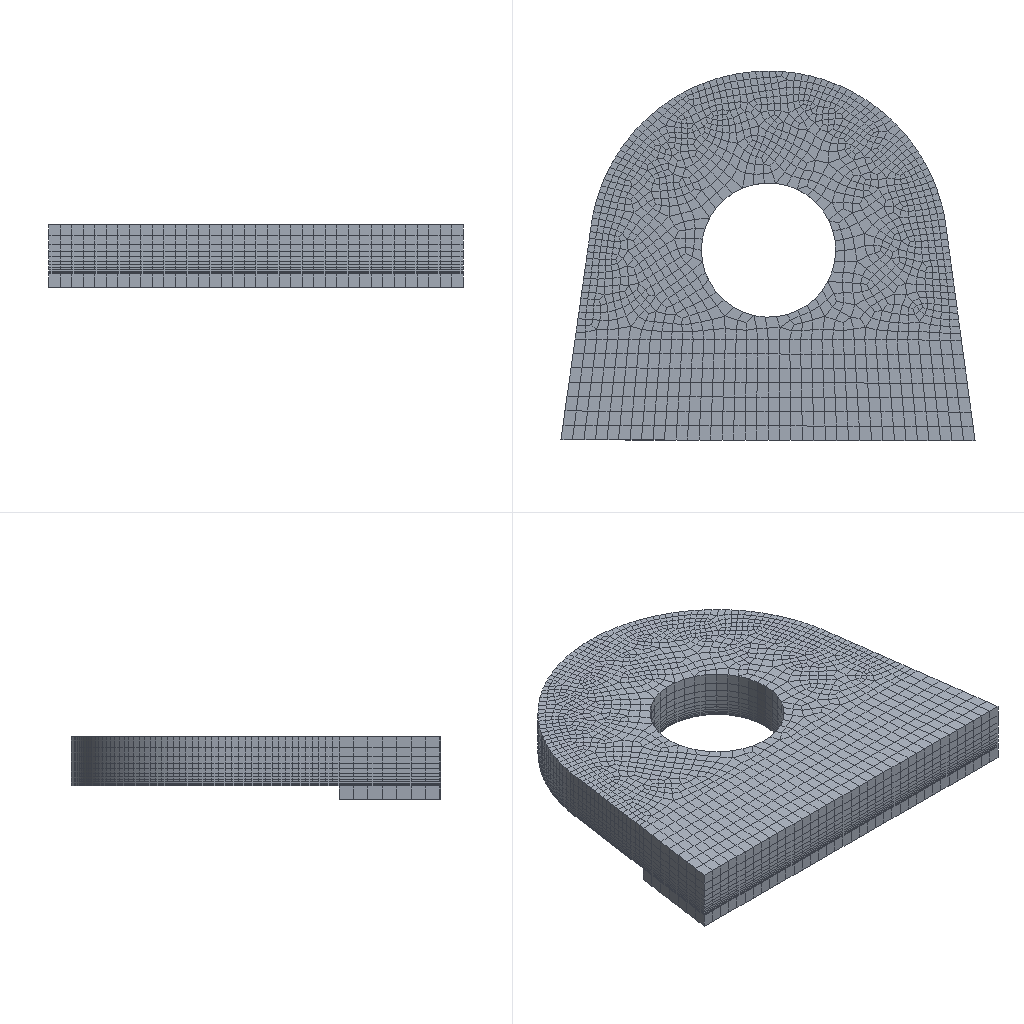Simulation study | abaqus
Set-up summary:
category,name,step,type,value,unit,region
solver,abaqus
solver,version,,,Abaqus/Explicit 2020
units,not stated in the deck,,not stated
analysis,deck,,transient,transient
load_step,Step-1,Step-1,transient
load_step,requested,,,1
mesh,nodes,,,20642
mesh,elements,,,17959
element_type,R3D3,,rigid,72
element_type,R3D4,,rigid,1311
element_type,C3D8R,,solid,16576
load,load commands in deck,,count,2
bc,support commands in deck,,count,7
material,MATERIAL-1,,in results
check,setup vs results,,match,"per instance, exact: element labels, types and connectivity; labels of the nodes the elements use; coordinates of those nodes at SINGLE_PRECISION in 1 of 2 instance(s)"
Abaqus input file, long lists of numbers shortened:
*Heading
** Job name: Job-1 Model name: Model-1
** Generated by: Abaqus/CAE 2020
*Preprint, echo=NO, model=NO, history=NO, contact=NO
**
** PARTS
**
*Part, name=work-1
*Node
      1,  -42.966,   51.411,  -25.061
      2,  -42.139,   50.996,  -24.866
** (1347 more lines like these left out)
*Element, type=R3D4
 1,   1,  25, 357,  62
 2,  25,   2,  26, 357
** (1309 more lines like these left out)
*Element, type=R3D3
39, 75,  5, 63
55,   9,  76, 143
** (70 more lines like these left out)
*Node
   1350,  -37.888,   63.4,  -26.953
*Nset, nset=work-1-RefPt_, internal
1350,
*Elset, elset=work-1, generate
    1,  1383,     1
*End Part
**
*Part, name=work-2
*Node
      1,  -25.624,   43.005,  -23.952
      2,  -27.048,   38.691,  -23.952
** (19290 more lines like these left out)
*Element, type=C3D8R
  1, 112, 568, 778,  43,   1,  19,  30,   4
  2, 568, 569, 779, 778,  19,  20,  29,  30
** (16574 more lines like these left out)
*Nset, nset=Set-1, generate
     1,  19292,      1
*Elset, elset=Set-1, generate
     1,  16576,      1
** Section: Section-1
*Solid Section, elset=Set-1, material=Material-1
,
*End Part
**
**
** ASSEMBLY
**
*Assembly, name=Assembly
**
*Instance, name=work-1-1, part=work-1
41.272, -22.918,    25.552
41.272, -22.918,    25.552, 41.272, -22.918, 26.552, 26.
*End Instance
**
*Instance, name=work-2-1, part=work-2
41.272, -22.918,    24.552
41.272, -22.918,    24.552, 41.272, -22.918, 25.552, 26.
*End Instance
**
*Nset, nset=Set-2, instance=work-2-1
    2,    3,    5,    6,   15,   16,  113,  114,  115,  116,  117,  118,  119,  120,  121,  122
  123,  124,  125,  126,  127,  128,  129,  130,  131,  132,  133,  134,  135,  136,  137,  138
** (29 more lines like these left out)
*Elset, elset=Set-2, instance=work-2-1
     7,    14,    21,    28,    35,    42,    49,    56,    63,    70,    77,    84,    91,    98,   105,   112
   119,   126,   133,   140,   147,   154,   161,   168,   175,   182,   189,   196,   203,   210,   217,   224
** (25 more lines like these left out)
*Nset, nset=Set-3, instance=work-1-1
 1350,
*Nset, nset=s_Set-1, instance=work-2-1
     1,     2,     5,     8,     9,    10,    11,    12,    13,    14,    15,    16,    17,    18,    19,    20
    21,    22,    23,    24,    31,    32,    33,    34,    35,    36,    78,    79,    80,    81,    82,    83
** (1186 more lines like these left out)
*Elset, elset=s_Set-1, instance=work-2-1, generate
   253,  16576,      1
*Elset, elset=_m_Surf-1_SPOS, internal, instance=work-1-1, generate
    1,  1383,     1
*Surface, type=ELEMENT, name=m_Surf-1
_m_Surf-1_SPOS, SPOS
*Surface, type=NODE, name=s_Set-1_CNS_, internal
s_Set-1, 1.
*Rigid Body, ref node=work-1-1.work-1-RefPt_, elset=work-1-1.work-1
*End Assembly
**
** MATERIALS
**
*Material, name=Material-1
*Damage Initiation, criterion=SHEAR
 0.01,0.,0.
*Damage Evolution, type=DISPLACEMENT
 0.0001,
*Density
 7.8e-09,
*Elastic
206000., 0.3
*Plastic
350.,   0.
429., 0.12
**
** INTERACTION PROPERTIES
**
*Surface Interaction, name=IntProp-1
*Friction
 0.15,
*Surface Behavior, pressure-overclosure=HARD
** ----------------------------------------------------------------
**
** STEP: Step-1
**
*Step, name=Step-1, nlgeom=YES
*Dynamic, Explicit
, 0.1
*Bulk Viscosity
0.06, 1.2
** Mass Scaling: Semi-Automatic
**               Whole Model
*Fixed Mass Scaling, factor=5000.
**
** BOUNDARY CONDITIONS
**
** Name: BC-1 Type: 对称/反对称/完全固定
*Boundary
Set-2, ENCASTRE
** Name: BC-2 Type: 速度/角速度
*Boundary, type=VELOCITY
Set-3, 1, 1, 180.
Set-3, 2, 2
Set-3, 3, 3
Set-3, 4, 4
Set-3, 5, 5, -628.
Set-3, 6, 6
**
** INTERACTIONS
**
** Interaction: Int-1
*Contact Pair, interaction=IntProp-1, mechanical constraint=KINEMATIC, cpset=Int-1
m_Surf-1, s_Set-1_CNS_
**
** OUTPUT REQUESTS
**
*Restart, write, number interval=1, time marks=NO
**
** FIELD OUTPUT: F-Output-1
**
*Output, field, number interval=50
*Node Output
A, CF, RF, RM, RT, U, V
*Element Output, directions=YES
E, EVF, LE, MISES, MISESMAX, MISESONLY, PE, PEEQ, PEEQMAX, PEEQT, PEEQVAVG, PEMAG, PEVAVG, S, SSAVG, STATUS
SVAVG, YIELDPOT
*Contact Output
CDISP, CSTRESS
**
** HISTORY OUTPUT: H-Output-1
**
*Output, history, time interval=2e-06
*Node Output, nset=Set-3
RF1, RF2, RF3
*End Step
Results summary:
result,step,Step-1,completed,increments=174887 time=0.1/0.1
result,analysis,,,transient
result,last_loadstep,,,1
result,primary field,,,U
result,reaction total,,FX,112.191,model units
result,reaction total,,FY,-178.221,model units
result,reaction total,,FZ,57.7,model units